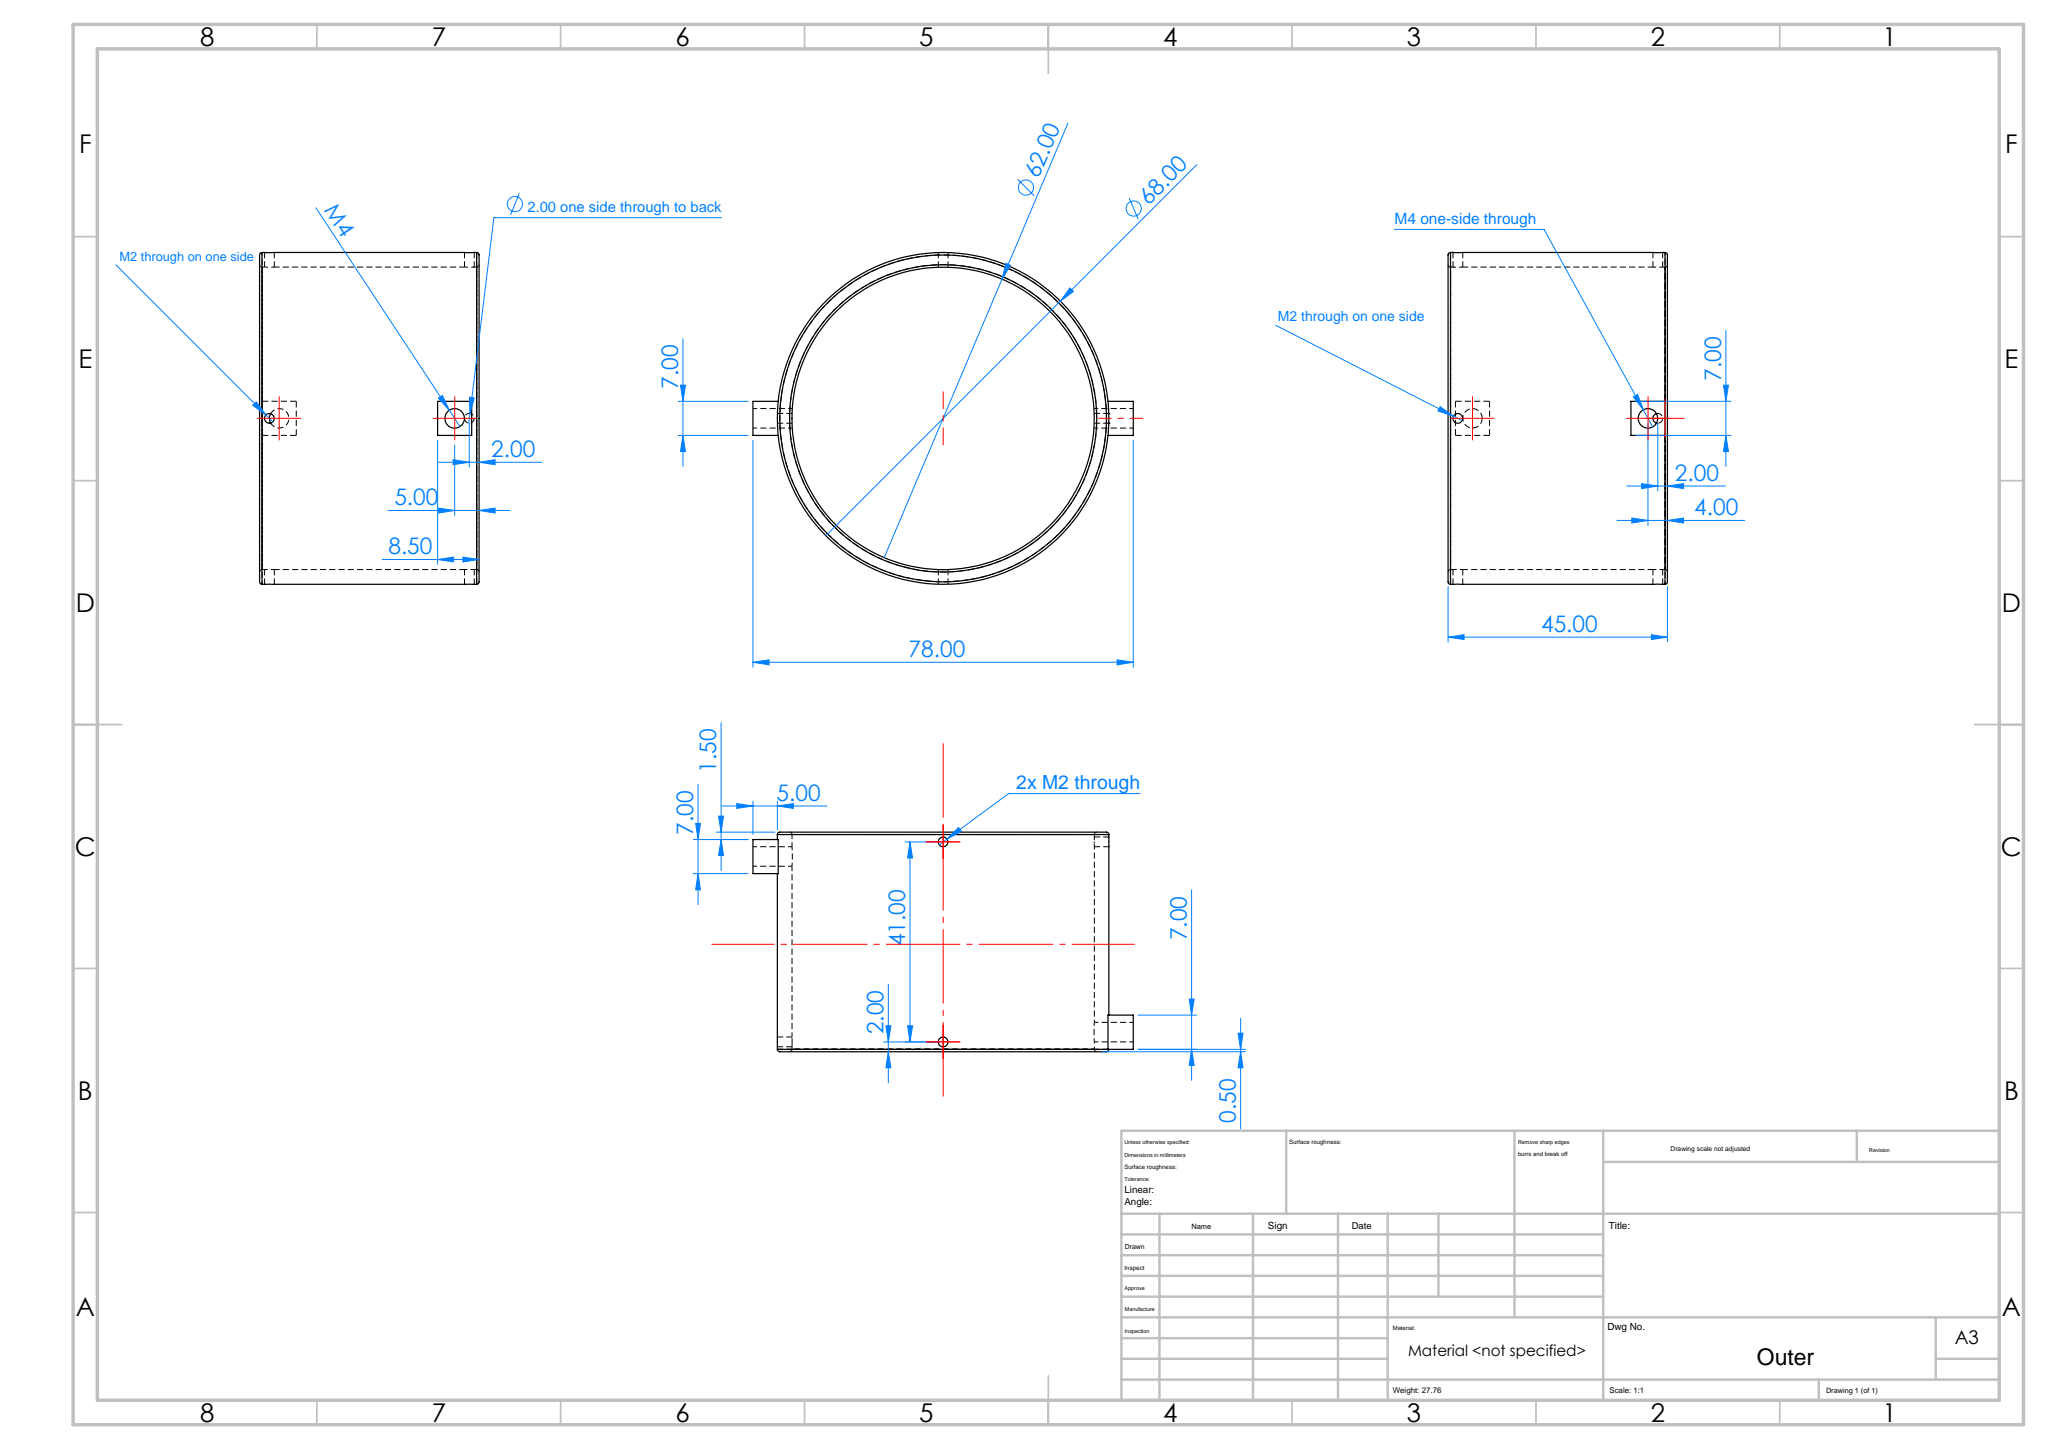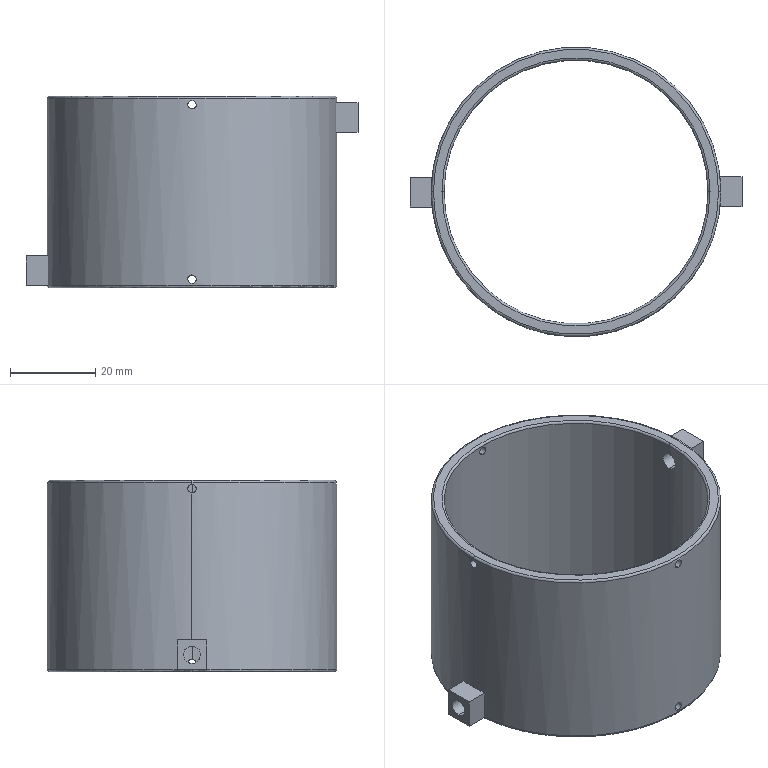Part | SolidWorks | features ICE 6, Fillet 3, CirPattern 2, Revolution 1 | 1 solid | 40 faces | box 78 x 68 x 45 mm | volume 27762 mm3 | cylinder 20 | plane 12 | torus 8 | commonest cylinder face diameters 2 x12 4 x4 62 x2 68 x2